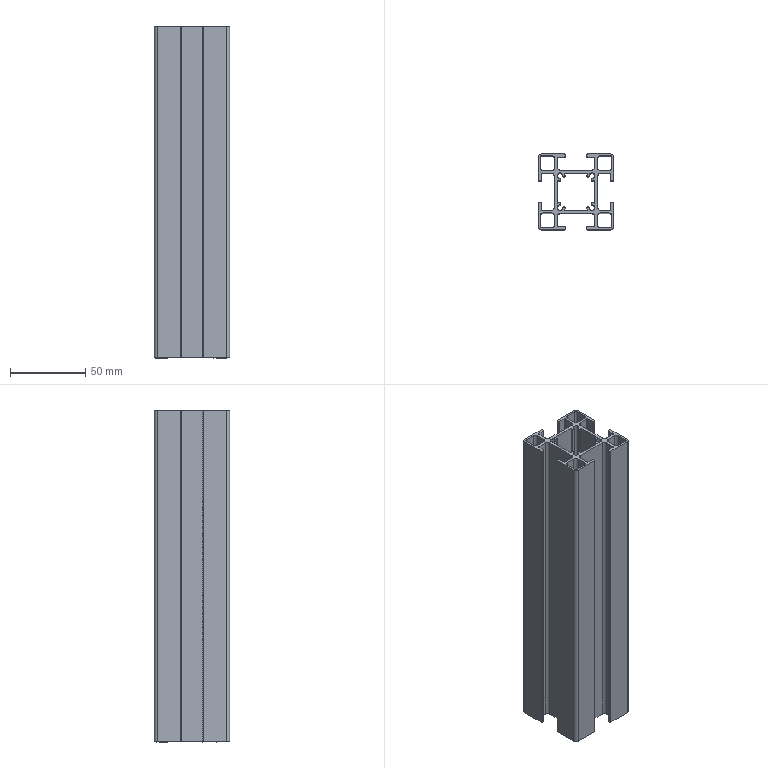Part | STEP file | 46A-00006CC11-220mm | 1 solid | 142 faces | box 50 x 50 x 220 mm | volume 129248 mm3 | cylinder 84 | plane 58 | commonest cylinder face diameters 1 x24 4 x24 1.5 x16 3.7 x8 6.7 x8 2 x4